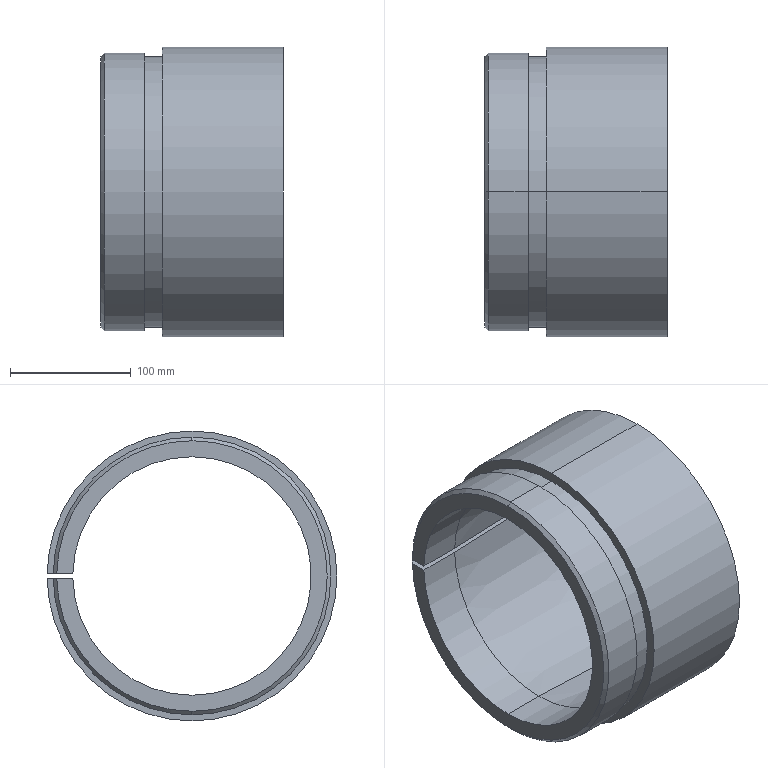Part | SolidWorks | features Chamfer 1, ICE 1, Revolution 1 | 1 solid | 24 faces | box 151 x 239.983 x 240 mm | volume 1801757 mm3 | cylinder 12 | cone 6 | plane 6 | commonest cylinder face diameters 197.4 x3 224 x3 230 x3 240 x3
STEP:
#1=CARTESIAN_POINT('',(0.,0.,112.));
#2=VERTEX_POINT('',#1);
#3=CARTESIAN_POINT('',(0.,111.982,2.));
#4=VERTEX_POINT('',#3);
#5=CARTESIAN_POINT('',(0.,0.,0.));
#6=DIRECTION('',(-1.,0.,0.));
#7=DIRECTION('',(0.,0.,-1.));
#8=AXIS2_PLACEMENT_3D('',#5,#6,#7);
#9=CIRCLE('',#8,112.);
#10=EDGE_CURVE('',#2,#4,#9,.T.);
#11=ORIENTED_EDGE('',*,*,#10,.F.);
#12=CARTESIAN_POINT('',(3.,0.,115.));
#13=VERTEX_POINT('',#12);
#14=CARTESIAN_POINT('',(0.,0.,112.));
#15=DIRECTION('',(0.7071,0.,0.7071));
#16=VECTOR('',#15,1000.);
#17=LINE('',#14,#16);
#18=EDGE_CURVE('',#2,#13,#17,.T.);
#19=ORIENTED_EDGE('',*,*,#18,.T.);
#20=CARTESIAN_POINT('',(3.,114.983,2.));
#21=VERTEX_POINT('',#20);
#22=CARTESIAN_POINT('',(3.,0.,0.));
#23=DIRECTION('',(1.,0.,0.));
#24=DIRECTION('',(0.,0.,-1.));
#25=AXIS2_PLACEMENT_3D('',#22,#23,#24);
#26=CIRCLE('',#25,115.);
#27=EDGE_CURVE('',#21,#13,#26,.T.);
#28=ORIENTED_EDGE('',*,*,#27,.F.);
#29=CARTESIAN_POINT('',(3.,114.983,2.));
#30=CARTESIAN_POINT('',(2.,113.982,2.));
#31=CARTESIAN_POINT('',(1.,112.982,2.));
#32=CARTESIAN_POINT('',(0.,111.982,2.));
#33=B_SPLINE_CURVE_WITH_KNOTS('',3,(#29,#30,#31,#32),.UNSPECIFIED.,.F.,.F.,(4,4),(0.07935,0.08359),.UNSPECIFIED.);
#34=EDGE_CURVE('',#21,#4,#33,.T.);
#35=ORIENTED_EDGE('',*,*,#34,.T.);
#36=EDGE_LOOP('',(#11,#19,#28,#35));
#37=FACE_OUTER_BOUND('',#36,.T.);
#38=CARTESIAN_POINT('',(0.,0.,0.));
#39=DIRECTION('',(1.,0.,0.));
#40=DIRECTION('',(0.,0.,-1.));
#41=AXIS2_PLACEMENT_3D('',#38,#39,#40);
#42=CONICAL_SURFACE('',#41,112.,0.7854);
#43=ADVANCED_FACE('',(#37),#42,.T.);
#44=ORIENTED_EDGE('',*,*,#18,.F.);
#45=CARTESIAN_POINT('',(0.,0.,-112.));
#46=VERTEX_POINT('',#45);
#47=CARTESIAN_POINT('',(0.,0.,0.));
#48=DIRECTION('',(-1.,0.,0.));
#49=DIRECTION('',(0.,0.,-1.));
#50=AXIS2_PLACEMENT_3D('',#47,#48,#49);
#51=CIRCLE('',#50,112.);
#52=EDGE_CURVE('',#46,#2,#51,.T.);
#53=ORIENTED_EDGE('',*,*,#52,.F.);
#54=CARTESIAN_POINT('',(3.,0.,-115.));
#55=VERTEX_POINT('',#54);
#56=CARTESIAN_POINT('',(0.,0.,-112.));
#57=DIRECTION('',(0.7071,0.,-0.7071));
#58=VECTOR('',#57,1000.);
#59=LINE('',#56,#58);
#60=EDGE_CURVE('',#46,#55,#59,.T.);
#61=ORIENTED_EDGE('',*,*,#60,.T.);
#62=CARTESIAN_POINT('',(3.,0.,0.));
#63=DIRECTION('',(1.,0.,0.));
#64=DIRECTION('',(0.,0.,-1.));
#65=AXIS2_PLACEMENT_3D('',#62,#63,#64);
#66=CIRCLE('',#65,115.);
#67=EDGE_CURVE('',#13,#55,#66,.T.);
#68=ORIENTED_EDGE('',*,*,#67,.F.);
#69=EDGE_LOOP('',(#44,#53,#61,#68));
#70=FACE_OUTER_BOUND('',#69,.T.);
#71=CARTESIAN_POINT('',(0.,0.,0.));
#72=DIRECTION('',(1.,0.,0.));
#73=DIRECTION('',(0.,0.,-1.));
#74=AXIS2_PLACEMENT_3D('',#71,#72,#73);
#75=CONICAL_SURFACE('',#74,112.,0.7854);
#76=ADVANCED_FACE('',(#70),#75,.T.);
#77=CARTESIAN_POINT('',(36.,0.,-98.7));
#78=VERTEX_POINT('',#77);
#79=CARTESIAN_POINT('',(36.,0.,98.7));
#80=VERTEX_POINT('',#79);
#81=CARTESIAN_POINT('',(36.,0.,0.));
#82=DIRECTION('',(-1.,0.,0.));
#83=DIRECTION('',(0.,0.,1.));
#84=AXIS2_PLACEMENT_3D('',#81,#82,#83);
#85=CIRCLE('',#84,98.7);
#86=EDGE_CURVE('',#78,#80,#85,.T.);
#87=ORIENTED_EDGE('',*,*,#86,.F.);
#88=CARTESIAN_POINT('',(0.,0.,-98.7));
#89=VERTEX_POINT('',#88);
#90=CARTESIAN_POINT('',(0.,0.,-98.7));
#91=DIRECTION('',(-1.,0.,0.));
#92=VECTOR('',#91,1000.);
#93=LINE('',#90,#92);
#94=EDGE_CURVE('',#78,#89,#93,.T.);
#95=ORIENTED_EDGE('',*,*,#94,.T.);
#96=CARTESIAN_POINT('',(0.,0.,98.7));
#97=VERTEX_POINT('',#96);
#98=CARTESIAN_POINT('',(0.,0.,0.));
#99=DIRECTION('',(-1.,0.,0.));
#100=DIRECTION('',(0.,0.,1.));
#101=AXIS2_PLACEMENT_3D('',#98,#99,#100);
#102=CIRCLE('',#101,98.7);
#103=EDGE_CURVE('',#89,#97,#102,.T.);
#104=ORIENTED_EDGE('',*,*,#103,.T.);
#105=CARTESIAN_POINT('',(0.,0.,98.7));
#106=DIRECTION('',(-1.,0.,0.));
#107=VECTOR('',#106,1000.);
#108=LINE('',#105,#107);
#109=EDGE_CURVE('',#80,#97,#108,.T.);
#110=ORIENTED_EDGE('',*,*,#109,.F.);
#111=EDGE_LOOP('',(#87,#95,#104,#110));
#112=FACE_OUTER_BOUND('',#111,.T.);
#113=CARTESIAN_POINT('',(0.,0.,0.));
#114=DIRECTION('',(-1.,0.,0.));
#115=DIRECTION('',(0.,0.,1.));
#116=AXIS2_PLACEMENT_3D('',#113,#114,#115);
#117=CYLINDRICAL_SURFACE('',#116,98.7);
#118=ADVANCED_FACE('',(#112),#117,.F.);
#119=CARTESIAN_POINT('',(36.,98.68,2.));
#120=VERTEX_POINT('',#119);
#121=CARTESIAN_POINT('',(36.,0.,0.));
#122=DIRECTION('',(-1.,0.,0.));
#123=DIRECTION('',(0.,0.,1.));
#124=AXIS2_PLACEMENT_3D('',#121,#122,#123);
#125=CIRCLE('',#124,98.7);
#126=EDGE_CURVE('',#80,#120,#125,.T.);
#127=ORIENTED_EDGE('',*,*,#126,.F.);
#128=ORIENTED_EDGE('',*,*,#109,.T.);
#129=CARTESIAN_POINT('',(0.,98.68,2.));
#130=VERTEX_POINT('',#129);
#131=CARTESIAN_POINT('',(0.,0.,0.));
#132=DIRECTION('',(-1.,0.,0.));
#133=DIRECTION('',(0.,0.,1.));
#134=AXIS2_PLACEMENT_3D('',#131,#132,#133);
#135=CIRCLE('',#134,98.7);
#136=EDGE_CURVE('',#97,#130,#135,.T.);
#137=ORIENTED_EDGE('',*,*,#136,.T.);
#138=CARTESIAN_POINT('',(0.,98.68,2.));
#139=DIRECTION('',(-1.,0.,0.));
#140=VECTOR('',#139,1000.);
#141=LINE('',#138,#140);
#142=EDGE_CURVE('',#120,#130,#141,.T.);
#143=ORIENTED_EDGE('',*,*,#142,.F.);
#144=EDGE_LOOP('',(#127,#128,#137,#143));
#145=FACE_OUTER_BOUND('',#144,.T.);
#146=CARTESIAN_POINT('',(0.,0.,0.));
#147=DIRECTION('',(-1.,0.,0.));
#148=DIRECTION('',(0.,0.,1.));
#149=AXIS2_PLACEMENT_3D('',#146,#147,#148);
#150=CYLINDRICAL_SURFACE('',#149,98.7);
#151=ADVANCED_FACE('',(#145),#150,.F.);
#152=ORIENTED_EDGE('',*,*,#86,.T.);
#153=CARTESIAN_POINT('',(151.,0.,103.5));
#154=VERTEX_POINT('',#153);
#155=CARTESIAN_POINT('',(36.,0.,98.7));
#156=DIRECTION('',(0.9991,0.,0.0417));
#157=VECTOR('',#156,1000.);
#158=LINE('',#155,#157);
#159=EDGE_CURVE('',#80,#154,#158,.T.);
#160=ORIENTED_EDGE('',*,*,#159,.T.);
#161=CARTESIAN_POINT('',(151.,0.,-103.5));
#162=VERTEX_POINT('',#161);
#163=CARTESIAN_POINT('',(151.,0.,0.));
#164=DIRECTION('',(-1.,0.,0.));
#165=DIRECTION('',(0.,0.,1.));
#166=AXIS2_PLACEMENT_3D('',#163,#164,#165);
#167=CIRCLE('',#166,103.5);
#168=EDGE_CURVE('',#162,#154,#167,.T.);
#169=ORIENTED_EDGE('',*,*,#168,.F.);
#170=CARTESIAN_POINT('',(36.,0.,-98.7));
#171=DIRECTION('',(0.9991,0.,-0.0417));
#172=VECTOR('',#171,1000.);
#173=LINE('',#170,#172);
#174=EDGE_CURVE('',#78,#162,#173,.T.);
#175=ORIENTED_EDGE('',*,*,#174,.F.);
#176=EDGE_LOOP('',(#152,#160,#169,#175));
#177=FACE_OUTER_BOUND('',#176,.T.);
#178=CARTESIAN_POINT('',(36.,0.,0.));
#179=DIRECTION('',(1.,0.,0.));
#180=DIRECTION('',(0.,0.,-1.));
#181=AXIS2_PLACEMENT_3D('',#178,#179,#180);
#182=CONICAL_SURFACE('',#181,98.7,0.04171);
#183=ADVANCED_FACE('',(#177),#182,.F.);
#184=CARTESIAN_POINT('',(36.,98.68,-2.));
#185=VERTEX_POINT('',#184);
#186=CARTESIAN_POINT('',(36.,0.,0.));
#187=DIRECTION('',(-1.,0.,0.));
#188=DIRECTION('',(0.,0.,1.));
#189=AXIS2_PLACEMENT_3D('',#186,#187,#188);
#190=CIRCLE('',#189,98.7);
#191=EDGE_CURVE('',#185,#78,#190,.T.);
#192=ORIENTED_EDGE('',*,*,#191,.T.);
#193=ORIENTED_EDGE('',*,*,#174,.T.);
#194=CARTESIAN_POINT('',(151.,103.481,-2.));
#195=VERTEX_POINT('',#194);
#196=CARTESIAN_POINT('',(151.,0.,0.));
#197=DIRECTION('',(-1.,0.,0.));
#198=DIRECTION('',(0.,0.,1.));
#199=AXIS2_PLACEMENT_3D('',#196,#197,#198);
#200=CIRCLE('',#199,103.5);
#201=EDGE_CURVE('',#195,#162,#200,.T.);
#202=ORIENTED_EDGE('',*,*,#201,.F.);
#203=CARTESIAN_POINT('',(36.,98.68,-2.));
#204=CARTESIAN_POINT('',(40.606,98.872,-2.));
#205=CARTESIAN_POINT('',(45.212,99.064,-2.));
#206=CARTESIAN_POINT('',(49.818,99.257,-2.));
#207=CARTESIAN_POINT('',(83.545,100.665,-2.));
#208=CARTESIAN_POINT('',(117.273,102.073,-2.));
#209=CARTESIAN_POINT('',(151.,103.481,-2.));
#210=B_SPLINE_CURVE_WITH_KNOTS('',3,(#203,#204,#205,#206,#207,#208,#209),.UNSPECIFIED.,.F.,.F.,(4,3,4),(0.1768,0.1906,0.2919),.UNSPECIFIED.);
#211=EDGE_CURVE('',#185,#195,#210,.T.);
#212=ORIENTED_EDGE('',*,*,#211,.F.);
#213=EDGE_LOOP('',(#192,#193,#202,#212));
#214=FACE_OUTER_BOUND('',#213,.T.);
#215=CARTESIAN_POINT('',(36.,0.,0.));
#216=DIRECTION('',(1.,0.,0.));
#217=DIRECTION('',(0.,0.,-1.));
#218=AXIS2_PLACEMENT_3D('',#215,#216,#217);
#219=CONICAL_SURFACE('',#218,98.7,0.04171);
#220=ADVANCED_FACE('',(#214),#219,.F.);
#221=CARTESIAN_POINT('',(151.,119.983,-2.));
#222=VERTEX_POINT('',#221);
#223=CARTESIAN_POINT('',(151.,0.,-120.));
#224=VERTEX_POINT('',#223);
#225=CARTESIAN_POINT('',(151.,0.,0.));
#226=DIRECTION('',(-1.,0.,0.));
#227=DIRECTION('',(0.,0.,1.));
#228=AXIS2_PLACEMENT_3D('',#225,#226,#227);
#229=CIRCLE('',#228,120.);
#230=EDGE_CURVE('',#222,#224,#229,.T.);
#231=ORIENTED_EDGE('',*,*,#230,.T.);
#232=CARTESIAN_POINT('',(51.,0.,-120.));
#233=VERTEX_POINT('',#232);
#234=CARTESIAN_POINT('',(0.,0.,-120.));
#235=DIRECTION('',(-1.,0.,0.));
#236=VECTOR('',#235,1000.);
#237=LINE('',#234,#236);
#238=EDGE_CURVE('',#224,#233,#237,.T.);
#239=ORIENTED_EDGE('',*,*,#238,.T.);
#240=CARTESIAN_POINT('',(51.,119.983,-2.));
#241=VERTEX_POINT('',#240);
#242=CARTESIAN_POINT('',(51.,0.,0.));
#243=DIRECTION('',(-1.,0.,0.));
#244=DIRECTION('',(0.,0.,1.));
#245=AXIS2_PLACEMENT_3D('',#242,#243,#244);
#246=CIRCLE('',#245,120.);
#247=EDGE_CURVE('',#241,#233,#246,.T.);
#248=ORIENTED_EDGE('',*,*,#247,.F.);
#249=CARTESIAN_POINT('',(0.,119.983,-2.));
#250=DIRECTION('',(-1.,0.,0.));
#251=VECTOR('',#250,1000.);
#252=LINE('',#249,#251);
#253=EDGE_CURVE('',#222,#241,#252,.T.);
#254=ORIENTED_EDGE('',*,*,#253,.F.);
#255=EDGE_LOOP('',(#231,#239,#248,#254));
#256=FACE_OUTER_BOUND('',#255,.T.);
#257=CARTESIAN_POINT('',(0.,0.,0.));
#258=DIRECTION('',(-1.,0.,0.));
#259=DIRECTION('',(0.,0.,1.));
#260=AXIS2_PLACEMENT_3D('',#257,#258,#259);
#261=CYLINDRICAL_SURFACE('',#260,120.);
#262=ADVANCED_FACE('',(#256),#261,.T.);
#263=ORIENTED_EDGE('',*,*,#238,.F.);
#264=CARTESIAN_POINT('',(151.,0.,120.));
#265=VERTEX_POINT('',#264);
#266=CARTESIAN_POINT('',(151.,0.,0.));
#267=DIRECTION('',(-1.,0.,0.));
#268=DIRECTION('',(0.,0.,1.));
#269=AXIS2_PLACEMENT_3D('',#266,#267,#268);
#270=CIRCLE('',#269,120.);
#271=EDGE_CURVE('',#224,#265,#270,.T.);
#272=ORIENTED_EDGE('',*,*,#271,.T.);
#273=CARTESIAN_POINT('',(51.,0.,120.));
#274=VERTEX_POINT('',#273);
#275=CARTESIAN_POINT('',(0.,0.,120.));
#276=DIRECTION('',(-1.,0.,0.));
#277=VECTOR('',#276,1000.);
#278=LINE('',#275,#277);
#279=EDGE_CURVE('',#265,#274,#278,.T.);
#280=ORIENTED_EDGE('',*,*,#279,.T.);
#281=CARTESIAN_POINT('',(51.,0.,0.));
#282=DIRECTION('',(-1.,0.,0.));
#283=DIRECTION('',(0.,0.,1.));
#284=AXIS2_PLACEMENT_3D('',#281,#282,#283);
#285=CIRCLE('',#284,120.);
#286=EDGE_CURVE('',#233,#274,#285,.T.);
#287=ORIENTED_EDGE('',*,*,#286,.F.);
#288=EDGE_LOOP('',(#263,#272,#280,#287));
#289=FACE_OUTER_BOUND('',#288,.T.);
#290=CARTESIAN_POINT('',(0.,0.,0.));
#291=DIRECTION('',(-1.,0.,0.));
#292=DIRECTION('',(0.,0.,1.));
#293=AXIS2_PLACEMENT_3D('',#290,#291,#292);
#294=CYLINDRICAL_SURFACE('',#293,120.);
#295=ADVANCED_FACE('',(#289),#294,.T.);
#296=CARTESIAN_POINT('',(51.,111.982,-2.));
#297=VERTEX_POINT('',#296);
#298=CARTESIAN_POINT('',(51.,0.,-112.));
#299=VERTEX_POINT('',#298);
#300=CARTESIAN_POINT('',(51.,0.,0.));
#301=DIRECTION('',(-1.,0.,0.));
#302=DIRECTION('',(0.,0.,1.));
#303=AXIS2_PLACEMENT_3D('',#300,#301,#302);
#304=CIRCLE('',#303,112.);
#305=EDGE_CURVE('',#297,#299,#304,.T.);
#306=ORIENTED_EDGE('',*,*,#305,.T.);
#307=CARTESIAN_POINT('',(36.,0.,-112.));
#308=VERTEX_POINT('',#307);
#309=CARTESIAN_POINT('',(0.,0.,-112.));
#310=DIRECTION('',(-1.,0.,0.));
#311=VECTOR('',#310,1000.);
#312=LINE('',#309,#311);
#313=EDGE_CURVE('',#299,#308,#312,.T.);
#314=ORIENTED_EDGE('',*,*,#313,.T.);
#315=CARTESIAN_POINT('',(36.,111.982,-2.));
#316=VERTEX_POINT('',#315);
#317=CARTESIAN_POINT('',(36.,0.,0.));
#318=DIRECTION('',(-1.,0.,0.));
#319=DIRECTION('',(0.,0.,1.));
#320=AXIS2_PLACEMENT_3D('',#317,#318,#319);
#321=CIRCLE('',#320,112.);
#322=EDGE_CURVE('',#316,#308,#321,.T.);
#323=ORIENTED_EDGE('',*,*,#322,.F.);
#324=CARTESIAN_POINT('',(0.,111.982,-2.));
#325=DIRECTION('',(-1.,0.,0.));
#326=VECTOR('',#325,1000.);
#327=LINE('',#324,#326);
#328=EDGE_CURVE('',#297,#316,#327,.T.);
#329=ORIENTED_EDGE('',*,*,#328,.F.);
#330=EDGE_LOOP('',(#306,#314,#323,#329));
#331=FACE_OUTER_BOUND('',#330,.T.);
#332=CARTESIAN_POINT('',(0.,0.,0.));
#333=DIRECTION('',(-1.,0.,0.));
#334=DIRECTION('',(0.,0.,1.));
#335=AXIS2_PLACEMENT_3D('',#332,#333,#334);
#336=CYLINDRICAL_SURFACE('',#335,112.);
#337=ADVANCED_FACE('',(#331),#336,.T.);
#338=ORIENTED_EDGE('',*,*,#313,.F.);
#339=CARTESIAN_POINT('',(51.,0.,112.));
#340=VERTEX_POINT('',#339);
#341=CARTESIAN_POINT('',(51.,0.,0.));
#342=DIRECTION('',(-1.,0.,0.));
#343=DIRECTION('',(0.,0.,1.));
#344=AXIS2_PLACEMENT_3D('',#341,#342,#343);
#345=CIRCLE('',#344,112.);
#346=EDGE_CURVE('',#299,#340,#345,.T.);
#347=ORIENTED_EDGE('',*,*,#346,.T.);
#348=CARTESIAN_POINT('',(36.,0.,112.));
#349=VERTEX_POINT('',#348);
#350=CARTESIAN_POINT('',(0.,0.,112.));
#351=DIRECTION('',(-1.,0.,0.));
#352=VECTOR('',#351,1000.);
#353=LINE('',#350,#352);
#354=EDGE_CURVE('',#340,#349,#353,.T.);
#355=ORIENTED_EDGE('',*,*,#354,.T.);
#356=CARTESIAN_POINT('',(36.,0.,0.));
#357=DIRECTION('',(-1.,0.,0.));
#358=DIRECTION('',(0.,0.,1.));
#359=AXIS2_PLACEMENT_3D('',#356,#357,#358);
#360=CIRCLE('',#359,112.);
#361=EDGE_CURVE('',#308,#349,#360,.T.);
#362=ORIENTED_EDGE('',*,*,#361,.F.);
#363=EDGE_LOOP('',(#338,#347,#355,#362));
#364=FACE_OUTER_BOUND('',#363,.T.);
#365=CARTESIAN_POINT('',(0.,0.,0.));
#366=DIRECTION('',(-1.,0.,0.));
#367=DIRECTION('',(0.,0.,1.));
#368=AXIS2_PLACEMENT_3D('',#365,#366,#367);
#369=CYLINDRICAL_SURFACE('',#368,112.);
#370=ADVANCED_FACE('',(#364),#369,.T.);
#371=CARTESIAN_POINT('',(36.,114.983,-2.));
#372=VERTEX_POINT('',#371);
#373=CARTESIAN_POINT('',(36.,0.,-115.));
#374=VERTEX_POINT('',#373);
#375=CARTESIAN_POINT('',(36.,0.,0.));
#376=DIRECTION('',(-1.,0.,0.));
#377=DIRECTION('',(0.,0.,1.));
#378=AXIS2_PLACEMENT_3D('',#375,#376,#377);
#379=CIRCLE('',#378,115.);
#380=EDGE_CURVE('',#372,#374,#379,.T.);
#381=ORIENTED_EDGE('',*,*,#380,.T.);
#382=CARTESIAN_POINT('',(0.,0.,-115.));
#383=DIRECTION('',(-1.,0.,0.));
#384=VECTOR('',#383,1000.);
#385=LINE('',#382,#384);
#386=EDGE_CURVE('',#374,#55,#385,.T.);
#387=ORIENTED_EDGE('',*,*,#386,.T.);
#388=CARTESIAN_POINT('',(3.,114.983,-2.));
#389=VERTEX_POINT('',#388);
#390=CARTESIAN_POINT('',(3.,0.,0.));
#391=DIRECTION('',(1.,0.,0.));
#392=DIRECTION('',(0.,0.,-1.));
#393=AXIS2_PLACEMENT_3D('',#390,#391,#392);
#394=CIRCLE('',#393,115.);
#395=EDGE_CURVE('',#55,#389,#394,.T.);
#396=ORIENTED_EDGE('',*,*,#395,.T.);
#397=CARTESIAN_POINT('',(0.,114.983,-2.));
#398=DIRECTION('',(-1.,0.,0.));
#399=VECTOR('',#398,1000.);
#400=LINE('',#397,#399);
#401=EDGE_CURVE('',#372,#389,#400,.T.);
#402=ORIENTED_EDGE('',*,*,#401,.F.);
#403=EDGE_LOOP('',(#381,#387,#396,#402));
#404=FACE_OUTER_BOUND('',#403,.T.);
#405=CARTESIAN_POINT('',(0.,0.,0.));
#406=DIRECTION('',(-1.,0.,0.));
#407=DIRECTION('',(0.,0.,1.));
#408=AXIS2_PLACEMENT_3D('',#405,#406,#407);
#409=CYLINDRICAL_SURFACE('',#408,115.);
#410=ADVANCED_FACE('',(#404),#409,.T.);
#411=ORIENTED_EDGE('',*,*,#386,.F.);
#412=CARTESIAN_POINT('',(36.,0.,115.));
#413=VERTEX_POINT('',#412);
#414=CARTESIAN_POINT('',(36.,0.,0.));
#415=DIRECTION('',(-1.,0.,0.));
#416=DIRECTION('',(0.,0.,1.));
#417=AXIS2_PLACEMENT_3D('',#414,#415,#416);
#418=CIRCLE('',#417,115.);
#419=EDGE_CURVE('',#374,#413,#418,.T.);
#420=ORIENTED_EDGE('',*,*,#419,.T.);
#421=CARTESIAN_POINT('',(0.,0.,115.));
#422=DIRECTION('',(-1.,0.,0.));
#423=VECTOR('',#422,1000.);
#424=LINE('',#421,#423);
#425=EDGE_CURVE('',#413,#13,#424,.T.);
#426=ORIENTED_EDGE('',*,*,#425,.T.);
#427=ORIENTED_EDGE('',*,*,#67,.T.);
#428=EDGE_LOOP('',(#411,#420,#426,#427));
#429=FACE_OUTER_BOUND('',#428,.T.);
#430=CARTESIAN_POINT('',(0.,0.,0.));
#431=DIRECTION('',(-1.,0.,0.));
#432=DIRECTION('',(0.,0.,1.));
#433=AXIS2_PLACEMENT_3D('',#430,#431,#432);
#434=CYLINDRICAL_SURFACE('',#433,115.);
#435=ADVANCED_FACE('',(#429),#434,.T.);
#436=CARTESIAN_POINT('',(0.,68.309,2.));
#437=DIRECTION('',(0.,-1.,0.));
#438=VECTOR('',#437,1000.);
#439=LINE('',#436,#438);
#440=EDGE_CURVE('',#4,#130,#439,.T.);
#441=ORIENTED_EDGE('',*,*,#440,.T.);
#442=ORIENTED_EDGE('',*,*,#136,.F.);
#443=ORIENTED_EDGE('',*,*,#103,.F.);
#444=CARTESIAN_POINT('',(0.,98.68,-2.));
#445=VERTEX_POINT('',#444);
#446=CARTESIAN_POINT('',(0.,0.,0.));
#447=DIRECTION('',(-1.,0.,0.));
#448=DIRECTION('',(0.,0.,1.));
#449=AXIS2_PLACEMENT_3D('',#446,#447,#448);
#450=CIRCLE('',#449,98.7);
#451=EDGE_CURVE('',#445,#89,#450,.T.);
#452=ORIENTED_EDGE('',*,*,#451,.F.);
#453=CARTESIAN_POINT('',(0.,111.982,-2.));
#454=VERTEX_POINT('',#453);
#455=CARTESIAN_POINT('',(0.,68.309,-2.));
#456=DIRECTION('',(0.,1.,0.));
#457=VECTOR('',#456,1000.);
#458=LINE('',#455,#457);
#459=EDGE_CURVE('',#445,#454,#458,.T.);
#460=ORIENTED_EDGE('',*,*,#459,.T.);
#461=CARTESIAN_POINT('',(0.,0.,0.));
#462=DIRECTION('',(-1.,0.,0.));
#463=DIRECTION('',(0.,0.,-1.));
#464=AXIS2_PLACEMENT_3D('',#461,#462,#463);
#465=CIRCLE('',#464,112.);
#466=EDGE_CURVE('',#454,#46,#465,.T.);
#467=ORIENTED_EDGE('',*,*,#466,.T.);
#468=ORIENTED_EDGE('',*,*,#52,.T.);
#469=ORIENTED_EDGE('',*,*,#10,.T.);
#470=EDGE_LOOP('',(#441,#442,#443,#452,#460,#467,#468,#469));
#471=FACE_OUTER_BOUND('',#470,.T.);
#472=CARTESIAN_POINT('',(0.,98.7,0.));
#473=DIRECTION('',(1.,0.,0.));
#474=DIRECTION('',(0.,0.,-1.));
#475=AXIS2_PLACEMENT_3D('',#472,#473,#474);
#476=PLANE('',#475);
#477=ADVANCED_FACE('',(#471),#476,.F.);
#478=ORIENTED_EDGE('',*,*,#425,.F.);
#479=CARTESIAN_POINT('',(36.,114.983,2.));
#480=VERTEX_POINT('',#479);
#481=CARTESIAN_POINT('',(36.,0.,0.));
#482=DIRECTION('',(-1.,0.,0.));
#483=DIRECTION('',(0.,0.,1.));
#484=AXIS2_PLACEMENT_3D('',#481,#482,#483);
#485=CIRCLE('',#484,115.);
#486=EDGE_CURVE('',#413,#480,#485,.T.);
#487=ORIENTED_EDGE('',*,*,#486,.T.);
#488=CARTESIAN_POINT('',(0.,114.983,2.));
#489=DIRECTION('',(1.,0.,0.));
#490=VECTOR('',#489,1000.);
#491=LINE('',#488,#490);
#492=EDGE_CURVE('',#21,#480,#491,.T.);
#493=ORIENTED_EDGE('',*,*,#492,.F.);
#494=ORIENTED_EDGE('',*,*,#27,.T.);
#495=EDGE_LOOP('',(#478,#487,#493,#494));
#496=FACE_OUTER_BOUND('',#495,.T.);
#497=CARTESIAN_POINT('',(0.,0.,0.));
#498=DIRECTION('',(-1.,0.,0.));
#499=DIRECTION('',(0.,0.,1.));
#500=AXIS2_PLACEMENT_3D('',#497,#498,#499);
#501=CYLINDRICAL_SURFACE('',#500,115.);
#502=ADVANCED_FACE('',(#496),#501,.T.);
#503=CARTESIAN_POINT('',(36.,111.982,2.));
#504=VERTEX_POINT('',#503);
#505=CARTESIAN_POINT('',(36.,115.,2.));
#506=DIRECTION('',(0.,-1.,0.));
#507=VECTOR('',#506,1000.);
#508=LINE('',#505,#507);
#509=EDGE_CURVE('',#480,#504,#508,.T.);
#510=ORIENTED_EDGE('',*,*,#509,.F.);
#511=ORIENTED_EDGE('',*,*,#486,.F.);
#512=ORIENTED_EDGE('',*,*,#419,.F.);
#513=ORIENTED_EDGE('',*,*,#380,.F.);
#514=CARTESIAN_POINT('',(36.,115.,-2.));
#515=DIRECTION('',(0.,1.,0.));
#516=VECTOR('',#515,1000.);
#517=LINE('',#514,#516);
#518=EDGE_CURVE('',#316,#372,#517,.T.);
#519=ORIENTED_EDGE('',*,*,#518,.F.);
#520=ORIENTED_EDGE('',*,*,#322,.T.);
#521=ORIENTED_EDGE('',*,*,#361,.T.);
#522=CARTESIAN_POINT('',(36.,0.,0.));
#523=DIRECTION('',(-1.,0.,0.));
#524=DIRECTION('',(0.,0.,1.));
#525=AXIS2_PLACEMENT_3D('',#522,#523,#524);
#526=CIRCLE('',#525,112.);
#527=EDGE_CURVE('',#349,#504,#526,.T.);
#528=ORIENTED_EDGE('',*,*,#527,.T.);
#529=EDGE_LOOP('',(#510,#511,#512,#513,#519,#520,#521,#528));
#530=FACE_OUTER_BOUND('',#529,.T.);
#531=CARTESIAN_POINT('',(36.,115.,0.));
#532=DIRECTION('',(-1.,0.,0.));
#533=DIRECTION('',(0.,0.,1.));
#534=AXIS2_PLACEMENT_3D('',#531,#532,#533);
#535=PLANE('',#534);
#536=ADVANCED_FACE('',(#530),#535,.F.);
#537=ORIENTED_EDGE('',*,*,#354,.F.);
#538=CARTESIAN_POINT('',(51.,111.982,2.));
#539=VERTEX_POINT('',#538);
#540=CARTESIAN_POINT('',(51.,0.,0.));
#541=DIRECTION('',(-1.,0.,0.));
#542=DIRECTION('',(0.,0.,1.));
#543=AXIS2_PLACEMENT_3D('',#540,#541,#542);
#544=CIRCLE('',#543,112.);
#545=EDGE_CURVE('',#340,#539,#544,.T.);
#546=ORIENTED_EDGE('',*,*,#545,.T.);
#547=CARTESIAN_POINT('',(0.,111.982,2.));
#548=DIRECTION('',(1.,0.,0.));
#549=VECTOR('',#548,1000.);
#550=LINE('',#547,#549);
#551=EDGE_CURVE('',#504,#539,#550,.T.);
#552=ORIENTED_EDGE('',*,*,#551,.F.);
#553=ORIENTED_EDGE('',*,*,#527,.F.);
#554=EDGE_LOOP('',(#537,#546,#552,#553));
#555=FACE_OUTER_BOUND('',#554,.T.);
#556=CARTESIAN_POINT('',(0.,0.,0.));
#557=DIRECTION('',(-1.,0.,0.));
#558=DIRECTION('',(0.,0.,1.));
#559=AXIS2_PLACEMENT_3D('',#556,#557,#558);
#560=CYLINDRICAL_SURFACE('',#559,112.);
#561=ADVANCED_FACE('',(#555),#560,.T.);
#562=CARTESIAN_POINT('',(51.,119.983,2.));
#563=VERTEX_POINT('',#562);
#564=CARTESIAN_POINT('',(51.,112.,2.));
#565=DIRECTION('',(0.,1.,0.));
#566=VECTOR('',#565,1000.);
#567=LINE('',#564,#566);
#568=EDGE_CURVE('',#539,#563,#567,.T.);
#569=ORIENTED_EDGE('',*,*,#568,.F.);
#570=ORIENTED_EDGE('',*,*,#545,.F.);
#571=ORIENTED_EDGE('',*,*,#346,.F.);
#572=ORIENTED_EDGE('',*,*,#305,.F.);
#573=CARTESIAN_POINT('',(51.,112.,-2.));
#574=DIRECTION('',(0.,-1.,0.));
#575=VECTOR('',#574,1000.);
#576=LINE('',#573,#575);
#577=EDGE_CURVE('',#241,#297,#576,.T.);
#578=ORIENTED_EDGE('',*,*,#577,.F.);
#579=ORIENTED_EDGE('',*,*,#247,.T.);
#580=ORIENTED_EDGE('',*,*,#286,.T.);
#581=CARTESIAN_POINT('',(51.,0.,0.));
#582=DIRECTION('',(-1.,0.,0.));
#583=DIRECTION('',(0.,0.,1.));
#584=AXIS2_PLACEMENT_3D('',#581,#582,#583);
#585=CIRCLE('',#584,120.);
#586=EDGE_CURVE('',#274,#563,#585,.T.);
#587=ORIENTED_EDGE('',*,*,#586,.T.);
#588=EDGE_LOOP('',(#569,#570,#571,#572,#578,#579,#580,#587));
#589=FACE_OUTER_BOUND('',#588,.T.);
#590=CARTESIAN_POINT('',(51.,112.,0.));
#591=DIRECTION('',(1.,0.,0.));
#592=DIRECTION('',(0.,0.,-1.));
#593=AXIS2_PLACEMENT_3D('',#590,#591,#592);
#594=PLANE('',#593);
#595=ADVANCED_FACE('',(#589),#594,.F.);
#596=ORIENTED_EDGE('',*,*,#279,.F.);
#597=CARTESIAN_POINT('',(151.,119.983,2.));
#598=VERTEX_POINT('',#597);
#599=CARTESIAN_POINT('',(151.,0.,0.));
#600=DIRECTION('',(-1.,0.,0.));
#601=DIRECTION('',(0.,0.,1.));
#602=AXIS2_PLACEMENT_3D('',#599,#600,#601);
#603=CIRCLE('',#602,120.);
#604=EDGE_CURVE('',#265,#598,#603,.T.);
#605=ORIENTED_EDGE('',*,*,#604,.T.);
#606=CARTESIAN_POINT('',(0.,119.983,2.));
#607=DIRECTION('',(1.,0.,0.));
#608=VECTOR('',#607,1000.);
#609=LINE('',#606,#608);
#610=EDGE_CURVE('',#563,#598,#609,.T.);
#611=ORIENTED_EDGE('',*,*,#610,.F.);
#612=ORIENTED_EDGE('',*,*,#586,.F.);
#613=EDGE_LOOP('',(#596,#605,#611,#612));
#614=FACE_OUTER_BOUND('',#613,.T.);
#615=CARTESIAN_POINT('',(0.,0.,0.));
#616=DIRECTION('',(-1.,0.,0.));
#617=DIRECTION('',(0.,0.,1.));
#618=AXIS2_PLACEMENT_3D('',#615,#616,#617);
#619=CYLINDRICAL_SURFACE('',#618,120.);
#620=ADVANCED_FACE('',(#614),#619,.T.);
#621=CARTESIAN_POINT('',(151.,103.481,2.));
#622=VERTEX_POINT('',#621);
#623=CARTESIAN_POINT('',(151.,68.309,2.));
#624=DIRECTION('',(0.,-1.,0.));
#625=VECTOR('',#624,1000.);
#626=LINE('',#623,#625);
#627=EDGE_CURVE('',#598,#622,#626,.T.);
#628=ORIENTED_EDGE('',*,*,#627,.F.);
#629=ORIENTED_EDGE('',*,*,#604,.F.);
#630=ORIENTED_EDGE('',*,*,#271,.F.);
#631=ORIENTED_EDGE('',*,*,#230,.F.);
#632=CARTESIAN_POINT('',(151.,68.309,-2.));
#633=DIRECTION('',(0.,1.,0.));
#634=VECTOR('',#633,1000.);
#635=LINE('',#632,#634);
#636=EDGE_CURVE('',#195,#222,#635,.T.);
#637=ORIENTED_EDGE('',*,*,#636,.F.);
#638=ORIENTED_EDGE('',*,*,#201,.T.);
#639=ORIENTED_EDGE('',*,*,#168,.T.);
#640=CARTESIAN_POINT('',(151.,0.,0.));
#641=DIRECTION('',(-1.,0.,0.));
#642=DIRECTION('',(0.,0.,1.));
#643=AXIS2_PLACEMENT_3D('',#640,#641,#642);
#644=CIRCLE('',#643,103.5);
#645=EDGE_CURVE('',#154,#622,#644,.T.);
#646=ORIENTED_EDGE('',*,*,#645,.T.);
#647=EDGE_LOOP('',(#628,#629,#630,#631,#637,#638,#639,#646));
#648=FACE_OUTER_BOUND('',#647,.T.);
#649=CARTESIAN_POINT('',(151.,120.,0.));
#650=DIRECTION('',(-1.,0.,0.));
#651=DIRECTION('',(0.,0.,1.));
#652=AXIS2_PLACEMENT_3D('',#649,#650,#651);
#653=PLANE('',#652);
#654=ADVANCED_FACE('',(#648),#653,.F.);
#655=ORIENTED_EDGE('',*,*,#159,.F.);
#656=ORIENTED_EDGE('',*,*,#126,.T.);
#657=CARTESIAN_POINT('',(151.,103.481,2.));
#658=CARTESIAN_POINT('',(117.273,102.073,2.));
#659=CARTESIAN_POINT('',(83.545,100.665,2.));
#660=CARTESIAN_POINT('',(49.818,99.257,2.));
#661=CARTESIAN_POINT('',(45.212,99.064,2.));
#662=CARTESIAN_POINT('',(40.606,98.872,2.));
#663=CARTESIAN_POINT('',(36.,98.68,2.));
#664=B_SPLINE_CURVE_WITH_KNOTS('',3,(#657,#658,#659,#660,#661,#662,#663),.UNSPECIFIED.,.F.,.F.,(4,3,4),(0.08933,0.1906,0.2044),.UNSPECIFIED.);
#665=EDGE_CURVE('',#622,#120,#664,.T.);
#666=ORIENTED_EDGE('',*,*,#665,.F.);
#667=ORIENTED_EDGE('',*,*,#645,.F.);
#668=EDGE_LOOP('',(#655,#656,#666,#667));
#669=FACE_OUTER_BOUND('',#668,.T.);
#670=CARTESIAN_POINT('',(36.,0.,0.));
#671=DIRECTION('',(1.,0.,0.));
#672=DIRECTION('',(0.,0.,-1.));
#673=AXIS2_PLACEMENT_3D('',#670,#671,#672);
#674=CONICAL_SURFACE('',#673,98.7,0.04171);
#675=ADVANCED_FACE('',(#669),#674,.F.);
#676=ORIENTED_EDGE('',*,*,#94,.F.);
#677=ORIENTED_EDGE('',*,*,#191,.F.);
#678=CARTESIAN_POINT('',(0.,98.68,-2.));
#679=DIRECTION('',(1.,0.,0.));
#680=VECTOR('',#679,1000.);
#681=LINE('',#678,#680);
#682=EDGE_CURVE('',#445,#185,#681,.T.);
#683=ORIENTED_EDGE('',*,*,#682,.F.);
#684=ORIENTED_EDGE('',*,*,#451,.T.);
#685=EDGE_LOOP('',(#676,#677,#683,#684));
#686=FACE_OUTER_BOUND('',#685,.T.);
#687=CARTESIAN_POINT('',(0.,0.,0.));
#688=DIRECTION('',(-1.,0.,0.));
#689=DIRECTION('',(0.,0.,1.));
#690=AXIS2_PLACEMENT_3D('',#687,#688,#689);
#691=CYLINDRICAL_SURFACE('',#690,98.7);
#692=ADVANCED_FACE('',(#686),#691,.F.);
#693=ORIENTED_EDGE('',*,*,#60,.F.);
#694=ORIENTED_EDGE('',*,*,#466,.F.);
#695=CARTESIAN_POINT('',(0.,111.982,-2.));
#696=CARTESIAN_POINT('',(1.,112.982,-2.));
#697=CARTESIAN_POINT('',(2.,113.982,-2.));
#698=CARTESIAN_POINT('',(3.,114.983,-2.));
#699=B_SPLINE_CURVE_WITH_KNOTS('',3,(#695,#696,#697,#698),.UNSPECIFIED.,.F.,.F.,(4,4),(0.08546,0.0897),.UNSPECIFIED.);
#700=EDGE_CURVE('',#454,#389,#699,.T.);
#701=ORIENTED_EDGE('',*,*,#700,.T.);
#702=ORIENTED_EDGE('',*,*,#395,.F.);
#703=EDGE_LOOP('',(#693,#694,#701,#702));
#704=FACE_OUTER_BOUND('',#703,.T.);
#705=CARTESIAN_POINT('',(0.,0.,0.));
#706=DIRECTION('',(1.,0.,0.));
#707=DIRECTION('',(0.,0.,-1.));
#708=AXIS2_PLACEMENT_3D('',#705,#706,#707);
#709=CONICAL_SURFACE('',#708,112.,0.7854);
#710=ADVANCED_FACE('',(#704),#709,.T.);
#711=ORIENTED_EDGE('',*,*,#211,.T.);
#712=ORIENTED_EDGE('',*,*,#636,.T.);
#713=ORIENTED_EDGE('',*,*,#253,.T.);
#714=ORIENTED_EDGE('',*,*,#577,.T.);
#715=ORIENTED_EDGE('',*,*,#328,.T.);
#716=ORIENTED_EDGE('',*,*,#518,.T.);
#717=ORIENTED_EDGE('',*,*,#401,.T.);
#718=ORIENTED_EDGE('',*,*,#700,.F.);
#719=ORIENTED_EDGE('',*,*,#459,.F.);
#720=ORIENTED_EDGE('',*,*,#682,.T.);
#721=EDGE_LOOP('',(#711,#712,#713,#714,#715,#716,#717,#718,#719,#720));
#722=FACE_OUTER_BOUND('',#721,.T.);
#723=CARTESIAN_POINT('',(151.,68.309,-2.));
#724=DIRECTION('',(0.,0.,1.));
#725=DIRECTION('',(1.,0.,0.));
#726=AXIS2_PLACEMENT_3D('',#723,#724,#725);
#727=PLANE('',#726);
#728=ADVANCED_FACE('',(#722),#727,.T.);
#729=ORIENTED_EDGE('',*,*,#665,.T.);
#730=ORIENTED_EDGE('',*,*,#142,.T.);
#731=ORIENTED_EDGE('',*,*,#440,.F.);
#732=ORIENTED_EDGE('',*,*,#34,.F.);
#733=ORIENTED_EDGE('',*,*,#492,.T.);
#734=ORIENTED_EDGE('',*,*,#509,.T.);
#735=ORIENTED_EDGE('',*,*,#551,.T.);
#736=ORIENTED_EDGE('',*,*,#568,.T.);
#737=ORIENTED_EDGE('',*,*,#610,.T.);
#738=ORIENTED_EDGE('',*,*,#627,.T.);
#739=EDGE_LOOP('',(#729,#730,#731,#732,#733,#734,#735,#736,#737,#738));
#740=FACE_OUTER_BOUND('',#739,.T.);
#741=CARTESIAN_POINT('',(151.,68.309,2.));
#742=DIRECTION('',(0.,0.,-1.));
#743=DIRECTION('',(-1.,0.,0.));
#744=AXIS2_PLACEMENT_3D('',#741,#742,#743);
#745=PLANE('',#744);
#746=ADVANCED_FACE('',(#740),#745,.T.);
#747=CLOSED_SHELL('',(#43,#76,#118,#151,#183,#220,#262,#295,#337,#370,#410,#435,#477,#502,#536,#561,#595,#620,#654,#675,#692,#710,#728,#746));
#748=MANIFOLD_SOLID_BREP('',#747);
#749=CARTESIAN_POINT('',(0.,0.,0.));
#750=DIRECTION('',(0.,0.,1.));
#751=DIRECTION('',(1.,0.,0.));
#752=AXIS2_PLACEMENT_3D('',#749,#750,#751);
#753=(LENGTH_UNIT()NAMED_UNIT(*)SI_UNIT(.MILLI.,.METRE.));
#754=UNCERTAINTY_MEASURE_WITH_UNIT(LENGTH_MEASURE(0.00001),#753,'','');
#755=(NAMED_UNIT(*)PLANE_ANGLE_UNIT()SI_UNIT($,.RADIAN.));
#756=(NAMED_UNIT(*)SI_UNIT($,.STERADIAN.)SOLID_ANGLE_UNIT());
#757=(GEOMETRIC_REPRESENTATION_CONTEXT(3)GLOBAL_UNCERTAINTY_ASSIGNED_CONTEXT((#754))GLOBAL_UNIT_ASSIGNED_CONTEXT((#753,#755,#756))REPRESENTATION_CONTEXT('',''));
#758=ADVANCED_BREP_SHAPE_REPRESENTATION('',(#748,#752),#757);